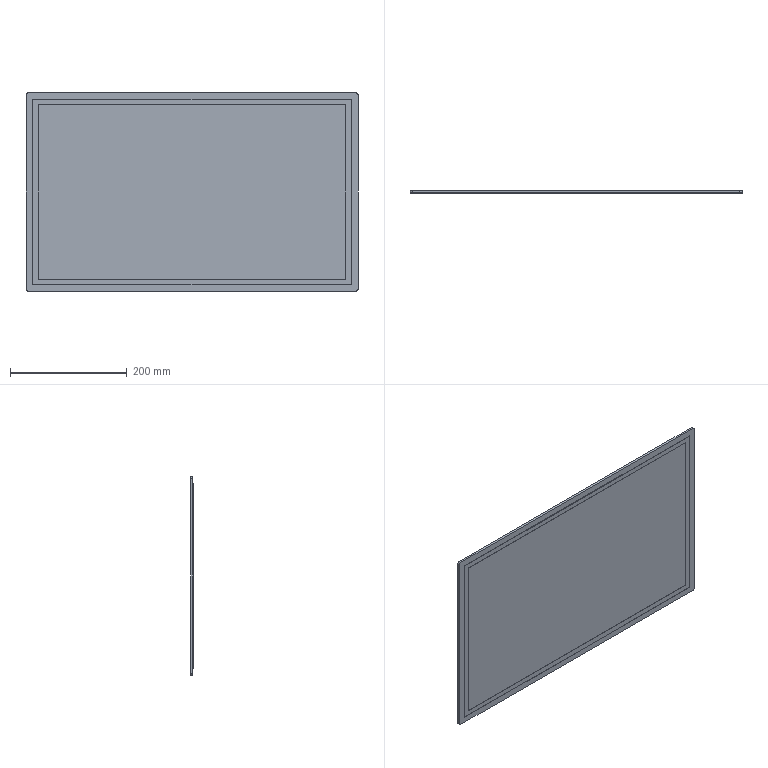Part | SolidWorks | features BaseBody 1 | 1 solid | 25 faces | box 569 x 4.9 x 340 mm | volume 738758 mm3 | plane 21 | cylinder 4 | commonest cylinder face diameters 7.4 x4
STEP:
#1=CARTESIAN_POINT('',(263.6,0.,149.6));
#2=VERTEX_POINT('',#1);
#3=CARTESIAN_POINT('',(263.6,0.,-149.6));
#4=VERTEX_POINT('',#3);
#5=CARTESIAN_POINT('',(263.6,0.,0.));
#6=DIRECTION('',(0.,0.,-1.));
#7=VECTOR('',#6,1000.);
#8=LINE('',#5,#7);
#9=EDGE_CURVE('',#2,#4,#8,.T.);
#10=ORIENTED_EDGE('',*,*,#9,.F.);
#11=CARTESIAN_POINT('',(-263.6,0.,149.6));
#12=VERTEX_POINT('',#11);
#13=CARTESIAN_POINT('',(0.,0.,149.6));
#14=DIRECTION('',(1.,0.,0.));
#15=VECTOR('',#14,1000.);
#16=LINE('',#13,#15);
#17=EDGE_CURVE('',#12,#2,#16,.T.);
#18=ORIENTED_EDGE('',*,*,#17,.F.);
#19=CARTESIAN_POINT('',(-263.6,0.,-149.6));
#20=VERTEX_POINT('',#19);
#21=CARTESIAN_POINT('',(-263.6,0.,0.));
#22=DIRECTION('',(0.,0.,1.));
#23=VECTOR('',#22,1000.);
#24=LINE('',#21,#23);
#25=EDGE_CURVE('',#20,#12,#24,.T.);
#26=ORIENTED_EDGE('',*,*,#25,.F.);
#27=CARTESIAN_POINT('',(0.,0.,-149.6));
#28=DIRECTION('',(-1.,0.,0.));
#29=VECTOR('',#28,1000.);
#30=LINE('',#27,#29);
#31=EDGE_CURVE('',#4,#20,#30,.T.);
#32=ORIENTED_EDGE('',*,*,#31,.F.);
#33=EDGE_LOOP('',(#10,#18,#26,#32));
#34=FACE_OUTER_BOUND('',#33,.T.);
#35=CARTESIAN_POINT('',(0.,0.,0.));
#36=DIRECTION('',(0.,1.,0.));
#37=DIRECTION('',(0.,0.,1.));
#38=AXIS2_PLACEMENT_3D('',#35,#36,#37);
#39=PLANE('',#38);
#40=ADVANCED_FACE('',(#34),#39,.F.);
#41=CARTESIAN_POINT('',(263.6,-1.,-149.6));
#42=VERTEX_POINT('',#41);
#43=CARTESIAN_POINT('',(263.6,0.,-149.6));
#44=DIRECTION('',(0.,1.,0.));
#45=VECTOR('',#44,1000.);
#46=LINE('',#43,#45);
#47=EDGE_CURVE('',#42,#4,#46,.T.);
#48=ORIENTED_EDGE('',*,*,#47,.T.);
#49=ORIENTED_EDGE('',*,*,#31,.T.);
#50=CARTESIAN_POINT('',(-263.6,-1.,-149.6));
#51=VERTEX_POINT('',#50);
#52=CARTESIAN_POINT('',(-263.6,0.,-149.6));
#53=DIRECTION('',(0.,-1.,0.));
#54=VECTOR('',#53,1000.);
#55=LINE('',#52,#54);
#56=EDGE_CURVE('',#20,#51,#55,.T.);
#57=ORIENTED_EDGE('',*,*,#56,.T.);
#58=CARTESIAN_POINT('',(263.6,-1.,-149.6));
#59=DIRECTION('',(1.,0.,0.));
#60=VECTOR('',#59,1000.);
#61=LINE('',#58,#60);
#62=EDGE_CURVE('',#51,#42,#61,.T.);
#63=ORIENTED_EDGE('',*,*,#62,.T.);
#64=EDGE_LOOP('',(#48,#49,#57,#63));
#65=FACE_OUTER_BOUND('',#64,.T.);
#66=CARTESIAN_POINT('',(263.6,0.,-149.6));
#67=DIRECTION('',(0.,0.,1.));
#68=DIRECTION('',(1.,0.,0.));
#69=AXIS2_PLACEMENT_3D('',#66,#67,#68);
#70=PLANE('',#69);
#71=ADVANCED_FACE('',(#65),#70,.T.);
#72=CARTESIAN_POINT('',(263.6,-1.,149.6));
#73=VERTEX_POINT('',#72);
#74=CARTESIAN_POINT('',(263.6,0.,149.6));
#75=DIRECTION('',(0.,1.,0.));
#76=VECTOR('',#75,1000.);
#77=LINE('',#74,#76);
#78=EDGE_CURVE('',#73,#2,#77,.T.);
#79=ORIENTED_EDGE('',*,*,#78,.T.);
#80=ORIENTED_EDGE('',*,*,#9,.T.);
#81=ORIENTED_EDGE('',*,*,#47,.F.);
#82=CARTESIAN_POINT('',(263.6,-1.,149.6));
#83=DIRECTION('',(0.,0.,1.));
#84=VECTOR('',#83,1000.);
#85=LINE('',#82,#84);
#86=EDGE_CURVE('',#42,#73,#85,.T.);
#87=ORIENTED_EDGE('',*,*,#86,.T.);
#88=EDGE_LOOP('',(#79,#80,#81,#87));
#89=FACE_OUTER_BOUND('',#88,.T.);
#90=CARTESIAN_POINT('',(263.6,0.,149.6));
#91=DIRECTION('',(-1.,0.,0.));
#92=DIRECTION('',(0.,0.,1.));
#93=AXIS2_PLACEMENT_3D('',#90,#91,#92);
#94=PLANE('',#93);
#95=ADVANCED_FACE('',(#89),#94,.T.);
#96=CARTESIAN_POINT('',(-263.6,-1.,149.6));
#97=VERTEX_POINT('',#96);
#98=CARTESIAN_POINT('',(-263.6,0.,149.6));
#99=DIRECTION('',(0.,1.,0.));
#100=VECTOR('',#99,1000.);
#101=LINE('',#98,#100);
#102=EDGE_CURVE('',#97,#12,#101,.T.);
#103=ORIENTED_EDGE('',*,*,#102,.T.);
#104=ORIENTED_EDGE('',*,*,#17,.T.);
#105=ORIENTED_EDGE('',*,*,#78,.F.);
#106=CARTESIAN_POINT('',(-263.6,-1.,149.6));
#107=DIRECTION('',(-1.,0.,0.));
#108=VECTOR('',#107,1000.);
#109=LINE('',#106,#108);
#110=EDGE_CURVE('',#73,#97,#109,.T.);
#111=ORIENTED_EDGE('',*,*,#110,.T.);
#112=EDGE_LOOP('',(#103,#104,#105,#111));
#113=FACE_OUTER_BOUND('',#112,.T.);
#114=CARTESIAN_POINT('',(-263.6,0.,149.6));
#115=DIRECTION('',(0.,0.,-1.));
#116=DIRECTION('',(-1.,0.,0.));
#117=AXIS2_PLACEMENT_3D('',#114,#115,#116);
#118=PLANE('',#117);
#119=ADVANCED_FACE('',(#113),#118,.T.);
#120=ORIENTED_EDGE('',*,*,#56,.F.);
#121=ORIENTED_EDGE('',*,*,#25,.T.);
#122=ORIENTED_EDGE('',*,*,#102,.F.);
#123=CARTESIAN_POINT('',(-263.6,-1.,-149.6));
#124=DIRECTION('',(0.,0.,-1.));
#125=VECTOR('',#124,1000.);
#126=LINE('',#123,#125);
#127=EDGE_CURVE('',#97,#51,#126,.T.);
#128=ORIENTED_EDGE('',*,*,#127,.T.);
#129=EDGE_LOOP('',(#120,#121,#122,#128));
#130=FACE_OUTER_BOUND('',#129,.T.);
#131=CARTESIAN_POINT('',(-263.6,0.,-149.6));
#132=DIRECTION('',(1.,0.,0.));
#133=DIRECTION('',(0.,0.,-1.));
#134=AXIS2_PLACEMENT_3D('',#131,#132,#133);
#135=PLANE('',#134);
#136=ADVANCED_FACE('',(#130),#135,.T.);
#137=ORIENTED_EDGE('',*,*,#62,.F.);
#138=ORIENTED_EDGE('',*,*,#127,.F.);
#139=ORIENTED_EDGE('',*,*,#110,.F.);
#140=ORIENTED_EDGE('',*,*,#86,.F.);
#141=EDGE_LOOP('',(#137,#138,#139,#140));
#142=FACE_BOUND('',#141,.T.);
#143=CARTESIAN_POINT('',(-272.6,-1.,-158.6));
#144=VERTEX_POINT('',#143);
#145=CARTESIAN_POINT('',(272.6,-1.,-158.6));
#146=VERTEX_POINT('',#145);
#147=CARTESIAN_POINT('',(0.,-1.,-158.6));
#148=DIRECTION('',(1.,0.,0.));
#149=VECTOR('',#148,1000.);
#150=LINE('',#147,#149);
#151=EDGE_CURVE('',#144,#146,#150,.T.);
#152=ORIENTED_EDGE('',*,*,#151,.T.);
#153=CARTESIAN_POINT('',(272.6,-1.,158.6));
#154=VERTEX_POINT('',#153);
#155=CARTESIAN_POINT('',(272.6,-1.,0.));
#156=DIRECTION('',(0.,0.,1.));
#157=VECTOR('',#156,1000.);
#158=LINE('',#155,#157);
#159=EDGE_CURVE('',#146,#154,#158,.T.);
#160=ORIENTED_EDGE('',*,*,#159,.T.);
#161=CARTESIAN_POINT('',(-272.6,-1.,158.6));
#162=VERTEX_POINT('',#161);
#163=CARTESIAN_POINT('',(0.,-1.,158.6));
#164=DIRECTION('',(-1.,0.,0.));
#165=VECTOR('',#164,1000.);
#166=LINE('',#163,#165);
#167=EDGE_CURVE('',#154,#162,#166,.T.);
#168=ORIENTED_EDGE('',*,*,#167,.T.);
#169=CARTESIAN_POINT('',(-272.6,-1.,0.));
#170=DIRECTION('',(0.,0.,-1.));
#171=VECTOR('',#170,1000.);
#172=LINE('',#169,#171);
#173=EDGE_CURVE('',#162,#144,#172,.T.);
#174=ORIENTED_EDGE('',*,*,#173,.T.);
#175=EDGE_LOOP('',(#152,#160,#168,#174));
#176=FACE_OUTER_BOUND('',#175,.T.);
#177=CARTESIAN_POINT('',(0.,-1.,0.));
#178=DIRECTION('',(0.,-1.,0.));
#179=DIRECTION('',(0.,0.,-1.));
#180=AXIS2_PLACEMENT_3D('',#177,#178,#179);
#181=PLANE('',#180);
#182=ADVANCED_FACE('',(#142,#176),#181,.T.);
#183=CARTESIAN_POINT('',(272.6,0.,-158.6));
#184=VERTEX_POINT('',#183);
#185=CARTESIAN_POINT('',(272.6,0.,-158.6));
#186=DIRECTION('',(0.,1.,0.));
#187=VECTOR('',#186,1000.);
#188=LINE('',#185,#187);
#189=EDGE_CURVE('',#146,#184,#188,.T.);
#190=ORIENTED_EDGE('',*,*,#189,.T.);
#191=CARTESIAN_POINT('',(272.6,0.,158.6));
#192=VERTEX_POINT('',#191);
#193=CARTESIAN_POINT('',(272.6,0.,-158.6));
#194=DIRECTION('',(0.,0.,1.));
#195=VECTOR('',#194,1000.);
#196=LINE('',#193,#195);
#197=EDGE_CURVE('',#184,#192,#196,.T.);
#198=ORIENTED_EDGE('',*,*,#197,.T.);
#199=CARTESIAN_POINT('',(272.6,0.,158.6));
#200=DIRECTION('',(0.,-1.,0.));
#201=VECTOR('',#200,1000.);
#202=LINE('',#199,#201);
#203=EDGE_CURVE('',#192,#154,#202,.T.);
#204=ORIENTED_EDGE('',*,*,#203,.T.);
#205=ORIENTED_EDGE('',*,*,#159,.F.);
#206=EDGE_LOOP('',(#190,#198,#204,#205));
#207=FACE_OUTER_BOUND('',#206,.T.);
#208=CARTESIAN_POINT('',(272.6,0.,-158.6));
#209=DIRECTION('',(1.,0.,0.));
#210=DIRECTION('',(0.,0.,-1.));
#211=AXIS2_PLACEMENT_3D('',#208,#209,#210);
#212=PLANE('',#211);
#213=ADVANCED_FACE('',(#207),#212,.T.);
#214=CARTESIAN_POINT('',(-272.6,0.,-158.6));
#215=VERTEX_POINT('',#214);
#216=CARTESIAN_POINT('',(-272.6,0.,-158.6));
#217=DIRECTION('',(0.,1.,0.));
#218=VECTOR('',#217,1000.);
#219=LINE('',#216,#218);
#220=EDGE_CURVE('',#144,#215,#219,.T.);
#221=ORIENTED_EDGE('',*,*,#220,.T.);
#222=CARTESIAN_POINT('',(-272.6,0.,-158.6));
#223=DIRECTION('',(1.,0.,0.));
#224=VECTOR('',#223,1000.);
#225=LINE('',#222,#224);
#226=EDGE_CURVE('',#215,#184,#225,.T.);
#227=ORIENTED_EDGE('',*,*,#226,.T.);
#228=ORIENTED_EDGE('',*,*,#189,.F.);
#229=ORIENTED_EDGE('',*,*,#151,.F.);
#230=EDGE_LOOP('',(#221,#227,#228,#229));
#231=FACE_OUTER_BOUND('',#230,.T.);
#232=CARTESIAN_POINT('',(-272.6,0.,-158.6));
#233=DIRECTION('',(0.,0.,-1.));
#234=DIRECTION('',(-1.,0.,0.));
#235=AXIS2_PLACEMENT_3D('',#232,#233,#234);
#236=PLANE('',#235);
#237=ADVANCED_FACE('',(#231),#236,.T.);
#238=CARTESIAN_POINT('',(-272.6,0.,158.6));
#239=VERTEX_POINT('',#238);
#240=CARTESIAN_POINT('',(-272.6,0.,158.6));
#241=DIRECTION('',(0.,1.,0.));
#242=VECTOR('',#241,1000.);
#243=LINE('',#240,#242);
#244=EDGE_CURVE('',#162,#239,#243,.T.);
#245=ORIENTED_EDGE('',*,*,#244,.T.);
#246=CARTESIAN_POINT('',(-272.6,0.,158.6));
#247=DIRECTION('',(0.,0.,-1.));
#248=VECTOR('',#247,1000.);
#249=LINE('',#246,#248);
#250=EDGE_CURVE('',#239,#215,#249,.T.);
#251=ORIENTED_EDGE('',*,*,#250,.T.);
#252=ORIENTED_EDGE('',*,*,#220,.F.);
#253=ORIENTED_EDGE('',*,*,#173,.F.);
#254=EDGE_LOOP('',(#245,#251,#252,#253));
#255=FACE_OUTER_BOUND('',#254,.T.);
#256=CARTESIAN_POINT('',(-272.6,0.,158.6));
#257=DIRECTION('',(-1.,0.,0.));
#258=DIRECTION('',(0.,0.,1.));
#259=AXIS2_PLACEMENT_3D('',#256,#257,#258);
#260=PLANE('',#259);
#261=ADVANCED_FACE('',(#255),#260,.T.);
#262=ORIENTED_EDGE('',*,*,#203,.F.);
#263=CARTESIAN_POINT('',(272.6,0.,158.6));
#264=DIRECTION('',(-1.,0.,0.));
#265=VECTOR('',#264,1000.);
#266=LINE('',#263,#265);
#267=EDGE_CURVE('',#192,#239,#266,.T.);
#268=ORIENTED_EDGE('',*,*,#267,.T.);
#269=ORIENTED_EDGE('',*,*,#244,.F.);
#270=ORIENTED_EDGE('',*,*,#167,.F.);
#271=EDGE_LOOP('',(#262,#268,#269,#270));
#272=FACE_OUTER_BOUND('',#271,.T.);
#273=CARTESIAN_POINT('',(272.6,0.,158.6));
#274=DIRECTION('',(0.,0.,1.));
#275=DIRECTION('',(1.,0.,0.));
#276=AXIS2_PLACEMENT_3D('',#273,#274,#275);
#277=PLANE('',#276);
#278=ADVANCED_FACE('',(#272),#277,.T.);
#279=ORIENTED_EDGE('',*,*,#250,.F.);
#280=ORIENTED_EDGE('',*,*,#267,.F.);
#281=ORIENTED_EDGE('',*,*,#197,.F.);
#282=ORIENTED_EDGE('',*,*,#226,.F.);
#283=EDGE_LOOP('',(#279,#280,#281,#282));
#284=FACE_BOUND('',#283,.T.);
#285=CARTESIAN_POINT('',(284.5,0.,-166.3));
#286=VERTEX_POINT('',#285);
#287=CARTESIAN_POINT('',(280.8,0.,-170.));
#288=VERTEX_POINT('',#287);
#289=CARTESIAN_POINT('',(280.8,0.,-166.3));
#290=DIRECTION('',(0.,1.,0.));
#291=DIRECTION('',(0.,0.,1.));
#292=AXIS2_PLACEMENT_3D('',#289,#290,#291);
#293=CIRCLE('',#292,3.7);
#294=EDGE_CURVE('',#286,#288,#293,.T.);
#295=ORIENTED_EDGE('',*,*,#294,.F.);
#296=CARTESIAN_POINT('',(284.5,0.,166.3));
#297=VERTEX_POINT('',#296);
#298=CARTESIAN_POINT('',(284.5,0.,0.));
#299=DIRECTION('',(0.,0.,-1.));
#300=VECTOR('',#299,1000.);
#301=LINE('',#298,#300);
#302=EDGE_CURVE('',#297,#286,#301,.T.);
#303=ORIENTED_EDGE('',*,*,#302,.F.);
#304=CARTESIAN_POINT('',(280.8,0.,170.));
#305=VERTEX_POINT('',#304);
#306=CARTESIAN_POINT('',(280.8,0.,166.3));
#307=DIRECTION('',(0.,1.,0.));
#308=DIRECTION('',(0.,0.,1.));
#309=AXIS2_PLACEMENT_3D('',#306,#307,#308);
#310=CIRCLE('',#309,3.7);
#311=EDGE_CURVE('',#305,#297,#310,.T.);
#312=ORIENTED_EDGE('',*,*,#311,.F.);
#313=CARTESIAN_POINT('',(-280.8,0.,170.));
#314=VERTEX_POINT('',#313);
#315=CARTESIAN_POINT('',(0.,0.,170.));
#316=DIRECTION('',(1.,0.,0.));
#317=VECTOR('',#316,1000.);
#318=LINE('',#315,#317);
#319=EDGE_CURVE('',#314,#305,#318,.T.);
#320=ORIENTED_EDGE('',*,*,#319,.F.);
#321=CARTESIAN_POINT('',(-284.5,0.,166.3));
#322=VERTEX_POINT('',#321);
#323=CARTESIAN_POINT('',(-280.8,0.,166.3));
#324=DIRECTION('',(0.,1.,0.));
#325=DIRECTION('',(0.,0.,1.));
#326=AXIS2_PLACEMENT_3D('',#323,#324,#325);
#327=CIRCLE('',#326,3.7);
#328=EDGE_CURVE('',#322,#314,#327,.T.);
#329=ORIENTED_EDGE('',*,*,#328,.F.);
#330=CARTESIAN_POINT('',(-284.5,0.,-166.3));
#331=VERTEX_POINT('',#330);
#332=CARTESIAN_POINT('',(-284.5,0.,0.));
#333=DIRECTION('',(0.,0.,1.));
#334=VECTOR('',#333,1000.);
#335=LINE('',#332,#334);
#336=EDGE_CURVE('',#331,#322,#335,.T.);
#337=ORIENTED_EDGE('',*,*,#336,.F.);
#338=CARTESIAN_POINT('',(-280.8,0.,-170.));
#339=VERTEX_POINT('',#338);
#340=CARTESIAN_POINT('',(-280.8,0.,-166.3));
#341=DIRECTION('',(0.,1.,0.));
#342=DIRECTION('',(0.,0.,1.));
#343=AXIS2_PLACEMENT_3D('',#340,#341,#342);
#344=CIRCLE('',#343,3.7);
#345=EDGE_CURVE('',#339,#331,#344,.T.);
#346=ORIENTED_EDGE('',*,*,#345,.F.);
#347=CARTESIAN_POINT('',(0.,0.,-170.));
#348=DIRECTION('',(-1.,0.,0.));
#349=VECTOR('',#348,1000.);
#350=LINE('',#347,#349);
#351=EDGE_CURVE('',#288,#339,#350,.T.);
#352=ORIENTED_EDGE('',*,*,#351,.F.);
#353=EDGE_LOOP('',(#295,#303,#312,#320,#329,#337,#346,#352));
#354=FACE_OUTER_BOUND('',#353,.T.);
#355=CARTESIAN_POINT('',(0.,0.,0.));
#356=DIRECTION('',(0.,1.,0.));
#357=DIRECTION('',(0.,0.,1.));
#358=AXIS2_PLACEMENT_3D('',#355,#356,#357);
#359=PLANE('',#358);
#360=ADVANCED_FACE('',(#284,#354),#359,.F.);
#361=CARTESIAN_POINT('',(280.8,3.9,-170.));
#362=VERTEX_POINT('',#361);
#363=CARTESIAN_POINT('',(280.8,0.,-170.));
#364=DIRECTION('',(0.,-1.,0.));
#365=VECTOR('',#364,1000.);
#366=LINE('',#363,#365);
#367=EDGE_CURVE('',#362,#288,#366,.T.);
#368=ORIENTED_EDGE('',*,*,#367,.T.);
#369=ORIENTED_EDGE('',*,*,#351,.T.);
#370=CARTESIAN_POINT('',(-280.8,3.9,-170.));
#371=VERTEX_POINT('',#370);
#372=CARTESIAN_POINT('',(-280.8,0.,-170.));
#373=DIRECTION('',(0.,1.,0.));
#374=VECTOR('',#373,1000.);
#375=LINE('',#372,#374);
#376=EDGE_CURVE('',#339,#371,#375,.T.);
#377=ORIENTED_EDGE('',*,*,#376,.T.);
#378=CARTESIAN_POINT('',(280.8,3.9,-170.));
#379=DIRECTION('',(1.,0.,0.));
#380=VECTOR('',#379,1000.);
#381=LINE('',#378,#380);
#382=EDGE_CURVE('',#371,#362,#381,.T.);
#383=ORIENTED_EDGE('',*,*,#382,.T.);
#384=EDGE_LOOP('',(#368,#369,#377,#383));
#385=FACE_OUTER_BOUND('',#384,.T.);
#386=CARTESIAN_POINT('',(280.8,0.,-170.));
#387=DIRECTION('',(0.,0.,-1.));
#388=DIRECTION('',(-1.,0.,0.));
#389=AXIS2_PLACEMENT_3D('',#386,#387,#388);
#390=PLANE('',#389);
#391=ADVANCED_FACE('',(#385),#390,.T.);
#392=CARTESIAN_POINT('',(284.5,3.9,-166.3));
#393=VERTEX_POINT('',#392);
#394=CARTESIAN_POINT('',(284.5,0.,-166.3));
#395=DIRECTION('',(0.,-1.,0.));
#396=VECTOR('',#395,1000.);
#397=LINE('',#394,#396);
#398=EDGE_CURVE('',#393,#286,#397,.T.);
#399=ORIENTED_EDGE('',*,*,#398,.T.);
#400=ORIENTED_EDGE('',*,*,#294,.T.);
#401=ORIENTED_EDGE('',*,*,#367,.F.);
#402=CARTESIAN_POINT('',(280.8,3.9,-166.3));
#403=DIRECTION('',(0.,-1.,0.));
#404=DIRECTION('',(0.,0.,1.));
#405=AXIS2_PLACEMENT_3D('',#402,#403,#404);
#406=CIRCLE('',#405,3.7);
#407=EDGE_CURVE('',#362,#393,#406,.T.);
#408=ORIENTED_EDGE('',*,*,#407,.T.);
#409=EDGE_LOOP('',(#399,#400,#401,#408));
#410=FACE_OUTER_BOUND('',#409,.T.);
#411=CARTESIAN_POINT('',(280.8,0.,-166.3));
#412=DIRECTION('',(0.,1.,0.));
#413=DIRECTION('',(0.,0.,1.));
#414=AXIS2_PLACEMENT_3D('',#411,#412,#413);
#415=CYLINDRICAL_SURFACE('',#414,3.7);
#416=ADVANCED_FACE('',(#410),#415,.T.);
#417=CARTESIAN_POINT('',(284.5,3.9,166.3));
#418=VERTEX_POINT('',#417);
#419=CARTESIAN_POINT('',(284.5,0.,166.3));
#420=DIRECTION('',(0.,-1.,0.));
#421=VECTOR('',#420,1000.);
#422=LINE('',#419,#421);
#423=EDGE_CURVE('',#418,#297,#422,.T.);
#424=ORIENTED_EDGE('',*,*,#423,.T.);
#425=ORIENTED_EDGE('',*,*,#302,.T.);
#426=ORIENTED_EDGE('',*,*,#398,.F.);
#427=CARTESIAN_POINT('',(284.5,3.9,166.3));
#428=DIRECTION('',(0.,0.,1.));
#429=VECTOR('',#428,1000.);
#430=LINE('',#427,#429);
#431=EDGE_CURVE('',#393,#418,#430,.T.);
#432=ORIENTED_EDGE('',*,*,#431,.T.);
#433=EDGE_LOOP('',(#424,#425,#426,#432));
#434=FACE_OUTER_BOUND('',#433,.T.);
#435=CARTESIAN_POINT('',(284.5,0.,166.3));
#436=DIRECTION('',(1.,0.,0.));
#437=DIRECTION('',(0.,0.,-1.));
#438=AXIS2_PLACEMENT_3D('',#435,#436,#437);
#439=PLANE('',#438);
#440=ADVANCED_FACE('',(#434),#439,.T.);
#441=CARTESIAN_POINT('',(280.8,3.9,170.));
#442=VERTEX_POINT('',#441);
#443=CARTESIAN_POINT('',(280.8,0.,170.));
#444=DIRECTION('',(0.,-1.,0.));
#445=VECTOR('',#444,1000.);
#446=LINE('',#443,#445);
#447=EDGE_CURVE('',#442,#305,#446,.T.);
#448=ORIENTED_EDGE('',*,*,#447,.T.);
#449=ORIENTED_EDGE('',*,*,#311,.T.);
#450=ORIENTED_EDGE('',*,*,#423,.F.);
#451=CARTESIAN_POINT('',(280.8,3.9,166.3));
#452=DIRECTION('',(0.,-1.,0.));
#453=DIRECTION('',(0.,0.,1.));
#454=AXIS2_PLACEMENT_3D('',#451,#452,#453);
#455=CIRCLE('',#454,3.7);
#456=EDGE_CURVE('',#418,#442,#455,.T.);
#457=ORIENTED_EDGE('',*,*,#456,.T.);
#458=EDGE_LOOP('',(#448,#449,#450,#457));
#459=FACE_OUTER_BOUND('',#458,.T.);
#460=CARTESIAN_POINT('',(280.8,0.,166.3));
#461=DIRECTION('',(0.,1.,0.));
#462=DIRECTION('',(0.,0.,1.));
#463=AXIS2_PLACEMENT_3D('',#460,#461,#462);
#464=CYLINDRICAL_SURFACE('',#463,3.7);
#465=ADVANCED_FACE('',(#459),#464,.T.);
#466=CARTESIAN_POINT('',(-280.8,3.9,170.));
#467=VERTEX_POINT('',#466);
#468=CARTESIAN_POINT('',(-280.8,0.,170.));
#469=DIRECTION('',(0.,-1.,0.));
#470=VECTOR('',#469,1000.);
#471=LINE('',#468,#470);
#472=EDGE_CURVE('',#467,#314,#471,.T.);
#473=ORIENTED_EDGE('',*,*,#472,.T.);
#474=ORIENTED_EDGE('',*,*,#319,.T.);
#475=ORIENTED_EDGE('',*,*,#447,.F.);
#476=CARTESIAN_POINT('',(-280.8,3.9,170.));
#477=DIRECTION('',(-1.,0.,0.));
#478=VECTOR('',#477,1000.);
#479=LINE('',#476,#478);
#480=EDGE_CURVE('',#442,#467,#479,.T.);
#481=ORIENTED_EDGE('',*,*,#480,.T.);
#482=EDGE_LOOP('',(#473,#474,#475,#481));
#483=FACE_OUTER_BOUND('',#482,.T.);
#484=CARTESIAN_POINT('',(-280.8,0.,170.));
#485=DIRECTION('',(0.,0.,1.));
#486=DIRECTION('',(1.,0.,0.));
#487=AXIS2_PLACEMENT_3D('',#484,#485,#486);
#488=PLANE('',#487);
#489=ADVANCED_FACE('',(#483),#488,.T.);
#490=CARTESIAN_POINT('',(-284.5,3.9,166.3));
#491=VERTEX_POINT('',#490);
#492=CARTESIAN_POINT('',(-284.5,0.,166.3));
#493=DIRECTION('',(0.,-1.,0.));
#494=VECTOR('',#493,1000.);
#495=LINE('',#492,#494);
#496=EDGE_CURVE('',#491,#322,#495,.T.);
#497=ORIENTED_EDGE('',*,*,#496,.T.);
#498=ORIENTED_EDGE('',*,*,#328,.T.);
#499=ORIENTED_EDGE('',*,*,#472,.F.);
#500=CARTESIAN_POINT('',(-280.8,3.9,166.3));
#501=DIRECTION('',(0.,-1.,0.));
#502=DIRECTION('',(0.,0.,1.));
#503=AXIS2_PLACEMENT_3D('',#500,#501,#502);
#504=CIRCLE('',#503,3.7);
#505=EDGE_CURVE('',#467,#491,#504,.T.);
#506=ORIENTED_EDGE('',*,*,#505,.T.);
#507=EDGE_LOOP('',(#497,#498,#499,#506));
#508=FACE_OUTER_BOUND('',#507,.T.);
#509=CARTESIAN_POINT('',(-280.8,0.,166.3));
#510=DIRECTION('',(0.,1.,0.));
#511=DIRECTION('',(0.,0.,1.));
#512=AXIS2_PLACEMENT_3D('',#509,#510,#511);
#513=CYLINDRICAL_SURFACE('',#512,3.7);
#514=ADVANCED_FACE('',(#508),#513,.T.);
#515=CARTESIAN_POINT('',(-284.5,3.9,-166.3));
#516=VERTEX_POINT('',#515);
#517=CARTESIAN_POINT('',(-284.5,0.,-166.3));
#518=DIRECTION('',(0.,-1.,0.));
#519=VECTOR('',#518,1000.);
#520=LINE('',#517,#519);
#521=EDGE_CURVE('',#516,#331,#520,.T.);
#522=ORIENTED_EDGE('',*,*,#521,.T.);
#523=ORIENTED_EDGE('',*,*,#336,.T.);
#524=ORIENTED_EDGE('',*,*,#496,.F.);
#525=CARTESIAN_POINT('',(-284.5,3.9,-166.3));
#526=DIRECTION('',(0.,0.,-1.));
#527=VECTOR('',#526,1000.);
#528=LINE('',#525,#527);
#529=EDGE_CURVE('',#491,#516,#528,.T.);
#530=ORIENTED_EDGE('',*,*,#529,.T.);
#531=EDGE_LOOP('',(#522,#523,#524,#530));
#532=FACE_OUTER_BOUND('',#531,.T.);
#533=CARTESIAN_POINT('',(-284.5,0.,-166.3));
#534=DIRECTION('',(-1.,0.,0.));
#535=DIRECTION('',(0.,0.,1.));
#536=AXIS2_PLACEMENT_3D('',#533,#534,#535);
#537=PLANE('',#536);
#538=ADVANCED_FACE('',(#532),#537,.T.);
#539=ORIENTED_EDGE('',*,*,#376,.F.);
#540=ORIENTED_EDGE('',*,*,#345,.T.);
#541=ORIENTED_EDGE('',*,*,#521,.F.);
#542=CARTESIAN_POINT('',(-280.8,3.9,-166.3));
#543=DIRECTION('',(0.,-1.,0.));
#544=DIRECTION('',(0.,0.,1.));
#545=AXIS2_PLACEMENT_3D('',#542,#543,#544);
#546=CIRCLE('',#545,3.7);
#547=EDGE_CURVE('',#516,#371,#546,.T.);
#548=ORIENTED_EDGE('',*,*,#547,.T.);
#549=EDGE_LOOP('',(#539,#540,#541,#548));
#550=FACE_OUTER_BOUND('',#549,.T.);
#551=CARTESIAN_POINT('',(-280.8,0.,-166.3));
#552=DIRECTION('',(0.,1.,0.));
#553=DIRECTION('',(0.,0.,1.));
#554=AXIS2_PLACEMENT_3D('',#551,#552,#553);
#555=CYLINDRICAL_SURFACE('',#554,3.7);
#556=ADVANCED_FACE('',(#550),#555,.T.);
#557=CARTESIAN_POINT('',(261.6,3.9,147.6));
#558=VERTEX_POINT('',#557);
#559=CARTESIAN_POINT('',(-261.6,3.9,147.6));
#560=VERTEX_POINT('',#559);
#561=CARTESIAN_POINT('',(0.,3.9,147.6));
#562=DIRECTION('',(-1.,0.,0.));
#563=VECTOR('',#562,1000.);
#564=LINE('',#561,#563);
#565=EDGE_CURVE('',#558,#560,#564,.T.);
#566=ORIENTED_EDGE('',*,*,#565,.T.);
#567=CARTESIAN_POINT('',(-261.6,3.9,-147.6));
#568=VERTEX_POINT('',#567);
#569=CARTESIAN_POINT('',(-261.6,3.9,0.));
#570=DIRECTION('',(0.,0.,-1.));
#571=VECTOR('',#570,1000.);
#572=LINE('',#569,#571);
#573=EDGE_CURVE('',#560,#568,#572,.T.);
#574=ORIENTED_EDGE('',*,*,#573,.T.);
#575=CARTESIAN_POINT('',(261.6,3.9,-147.6));
#576=VERTEX_POINT('',#575);
#577=CARTESIAN_POINT('',(0.,3.9,-147.6));
#578=DIRECTION('',(1.,0.,0.));
#579=VECTOR('',#578,1000.);
#580=LINE('',#577,#579);
#581=EDGE_CURVE('',#568,#576,#580,.T.);
#582=ORIENTED_EDGE('',*,*,#581,.T.);
#583=CARTESIAN_POINT('',(261.6,3.9,0.));
#584=DIRECTION('',(0.,0.,1.));
#585=VECTOR('',#584,1000.);
#586=LINE('',#583,#585);
#587=EDGE_CURVE('',#576,#558,#586,.T.);
#588=ORIENTED_EDGE('',*,*,#587,.T.);
#589=EDGE_LOOP('',(#566,#574,#582,#588));
#590=FACE_BOUND('',#589,.T.);
#591=ORIENTED_EDGE('',*,*,#382,.F.);
#592=ORIENTED_EDGE('',*,*,#547,.F.);
#593=ORIENTED_EDGE('',*,*,#529,.F.);
#594=ORIENTED_EDGE('',*,*,#505,.F.);
#595=ORIENTED_EDGE('',*,*,#480,.F.);
#596=ORIENTED_EDGE('',*,*,#456,.F.);
#597=ORIENTED_EDGE('',*,*,#431,.F.);
#598=ORIENTED_EDGE('',*,*,#407,.F.);
#599=EDGE_LOOP('',(#591,#592,#593,#594,#595,#596,#597,#598));
#600=FACE_OUTER_BOUND('',#599,.T.);
#601=CARTESIAN_POINT('',(0.,3.9,0.));
#602=DIRECTION('',(0.,1.,0.));
#603=DIRECTION('',(0.,0.,1.));
#604=AXIS2_PLACEMENT_3D('',#601,#602,#603);
#605=PLANE('',#604);
#606=ADVANCED_FACE('',(#590,#600),#605,.T.);
#607=CARTESIAN_POINT('',(-261.6,3.7,-147.6));
#608=VERTEX_POINT('',#607);
#609=CARTESIAN_POINT('',(-261.6,3.7,147.6));
#610=VERTEX_POINT('',#609);
#611=CARTESIAN_POINT('',(-261.6,3.7,-147.6));
#612=DIRECTION('',(0.,0.,1.));
#613=VECTOR('',#612,1000.);
#614=LINE('',#611,#613);
#615=EDGE_CURVE('',#608,#610,#614,.T.);
#616=ORIENTED_EDGE('',*,*,#615,.F.);
#617=CARTESIAN_POINT('',(-261.6,3.9,-147.6));
#618=DIRECTION('',(0.,-1.,0.));
#619=VECTOR('',#618,1000.);
#620=LINE('',#617,#619);
#621=EDGE_CURVE('',#568,#608,#620,.T.);
#622=ORIENTED_EDGE('',*,*,#621,.F.);
#623=ORIENTED_EDGE('',*,*,#573,.F.);
#624=CARTESIAN_POINT('',(-261.6,3.9,147.6));
#625=DIRECTION('',(0.,1.,0.));
#626=VECTOR('',#625,1000.);
#627=LINE('',#624,#626);
#628=EDGE_CURVE('',#610,#560,#627,.T.);
#629=ORIENTED_EDGE('',*,*,#628,.F.);
#630=EDGE_LOOP('',(#616,#622,#623,#629));
#631=FACE_OUTER_BOUND('',#630,.T.);
#632=CARTESIAN_POINT('',(-261.6,3.9,-147.6));
#633=DIRECTION('',(-1.,0.,0.));
#634=DIRECTION('',(0.,0.,1.));
#635=AXIS2_PLACEMENT_3D('',#632,#633,#634);
#636=PLANE('',#635);
#637=ADVANCED_FACE('',(#631),#636,.F.);
#638=CARTESIAN_POINT('',(261.6,3.7,147.6));
#639=VERTEX_POINT('',#638);
#640=CARTESIAN_POINT('',(-261.6,3.7,147.6));
#641=DIRECTION('',(1.,0.,0.));
#642=VECTOR('',#641,1000.);
#643=LINE('',#640,#642);
#644=EDGE_CURVE('',#610,#639,#643,.T.);
#645=ORIENTED_EDGE('',*,*,#644,.F.);
#646=ORIENTED_EDGE('',*,*,#628,.T.);
#647=ORIENTED_EDGE('',*,*,#565,.F.);
#648=CARTESIAN_POINT('',(261.6,3.9,147.6));
#649=DIRECTION('',(0.,1.,0.));
#650=VECTOR('',#649,1000.);
#651=LINE('',#648,#650);
#652=EDGE_CURVE('',#639,#558,#651,.T.);
#653=ORIENTED_EDGE('',*,*,#652,.F.);
#654=EDGE_LOOP('',(#645,#646,#647,#653));
#655=FACE_OUTER_BOUND('',#654,.T.);
#656=CARTESIAN_POINT('',(-261.6,3.9,147.6));
#657=DIRECTION('',(0.,0.,1.));
#658=DIRECTION('',(1.,0.,0.));
#659=AXIS2_PLACEMENT_3D('',#656,#657,#658);
#660=PLANE('',#659);
#661=ADVANCED_FACE('',(#655),#660,.F.);
#662=CARTESIAN_POINT('',(261.6,3.7,-147.6));
#663=VERTEX_POINT('',#662);
#664=CARTESIAN_POINT('',(261.6,3.7,147.6));
#665=DIRECTION('',(0.,0.,-1.));
#666=VECTOR('',#665,1000.);
#667=LINE('',#664,#666);
#668=EDGE_CURVE('',#639,#663,#667,.T.);
#669=ORIENTED_EDGE('',*,*,#668,.F.);
#670=ORIENTED_EDGE('',*,*,#652,.T.);
#671=ORIENTED_EDGE('',*,*,#587,.F.);
#672=CARTESIAN_POINT('',(261.6,3.9,-147.6));
#673=DIRECTION('',(0.,1.,0.));
#674=VECTOR('',#673,1000.);
#675=LINE('',#672,#674);
#676=EDGE_CURVE('',#663,#576,#675,.T.);
#677=ORIENTED_EDGE('',*,*,#676,.F.);
#678=EDGE_LOOP('',(#669,#670,#671,#677));
#679=FACE_OUTER_BOUND('',#678,.T.);
#680=CARTESIAN_POINT('',(261.6,3.9,147.6));
#681=DIRECTION('',(1.,0.,0.));
#682=DIRECTION('',(0.,0.,-1.));
#683=AXIS2_PLACEMENT_3D('',#680,#681,#682);
#684=PLANE('',#683);
#685=ADVANCED_FACE('',(#679),#684,.F.);
#686=CARTESIAN_POINT('',(261.6,3.7,-147.6));
#687=DIRECTION('',(-1.,0.,0.));
#688=VECTOR('',#687,1000.);
#689=LINE('',#686,#688);
#690=EDGE_CURVE('',#663,#608,#689,.T.);
#691=ORIENTED_EDGE('',*,*,#690,.F.);
#692=ORIENTED_EDGE('',*,*,#676,.T.);
#693=ORIENTED_EDGE('',*,*,#581,.F.);
#694=ORIENTED_EDGE('',*,*,#621,.T.);
#695=EDGE_LOOP('',(#691,#692,#693,#694));
#696=FACE_OUTER_BOUND('',#695,.T.);
#697=CARTESIAN_POINT('',(261.6,3.9,-147.6));
#698=DIRECTION('',(0.,0.,-1.));
#699=DIRECTION('',(-1.,0.,0.));
#700=AXIS2_PLACEMENT_3D('',#697,#698,#699);
#701=PLANE('',#700);
#702=ADVANCED_FACE('',(#696),#701,.F.);
#703=ORIENTED_EDGE('',*,*,#690,.T.);
#704=ORIENTED_EDGE('',*,*,#615,.T.);
#705=ORIENTED_EDGE('',*,*,#644,.T.);
#706=ORIENTED_EDGE('',*,*,#668,.T.);
#707=EDGE_LOOP('',(#703,#704,#705,#706));
#708=FACE_OUTER_BOUND('',#707,.T.);
#709=CARTESIAN_POINT('',(0.,3.7,0.));
#710=DIRECTION('',(0.,1.,0.));
#711=DIRECTION('',(0.,0.,1.));
#712=AXIS2_PLACEMENT_3D('',#709,#710,#711);
#713=PLANE('',#712);
#714=ADVANCED_FACE('',(#708),#713,.T.);
#715=CLOSED_SHELL('',(#40,#71,#95,#119,#136,#182,#213,#237,#261,#278,#360,#391,#416,#440,#465,#489,#514,#538,#556,#606,#637,#661,#685,#702,#714));
#716=MANIFOLD_SOLID_BREP('',#715);
#717=CARTESIAN_POINT('',(0.,0.,0.));
#718=DIRECTION('',(0.,0.,1.));
#719=DIRECTION('',(1.,0.,0.));
#720=AXIS2_PLACEMENT_3D('',#717,#718,#719);
#721=(LENGTH_UNIT()NAMED_UNIT(*)SI_UNIT(.MILLI.,.METRE.));
#722=UNCERTAINTY_MEASURE_WITH_UNIT(LENGTH_MEASURE(0.00001),#721,'','');
#723=(NAMED_UNIT(*)PLANE_ANGLE_UNIT()SI_UNIT($,.RADIAN.));
#724=(NAMED_UNIT(*)SI_UNIT($,.STERADIAN.)SOLID_ANGLE_UNIT());
#725=(GEOMETRIC_REPRESENTATION_CONTEXT(3)GLOBAL_UNCERTAINTY_ASSIGNED_CONTEXT((#722))GLOBAL_UNIT_ASSIGNED_CONTEXT((#721,#723,#724))REPRESENTATION_CONTEXT('',''));
#726=ADVANCED_BREP_SHAPE_REPRESENTATION('',(#716,#720),#725);